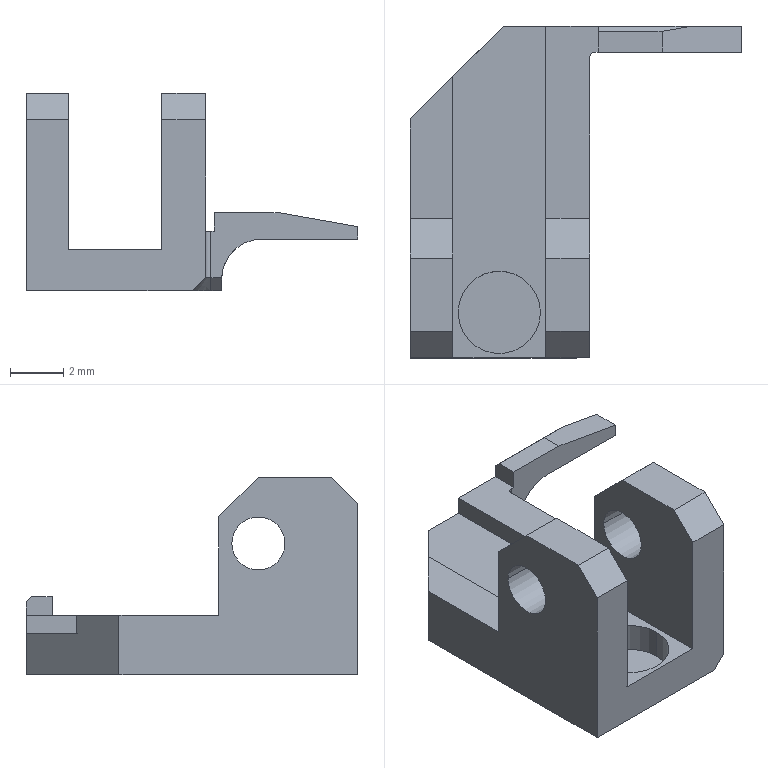Part | NX | 1 solid | 39 faces | box 12.481 x 12.5 x 7.45 mm | volume 216.351 mm3 | plane 30 | cylinder 8 | cone 1 | commonest cylinder face diameters 2 x4 3.1 x2 0.4 x1 3 x1
STEP:
#1=CARTESIAN_POINT('',(-42.479,-42.729,-0.8259));
#2=VERTEX_POINT('',#1);
#3=CARTESIAN_POINT('',(-42.479,-43.716,-0.8259));
#4=VERTEX_POINT('',#3);
#5=CARTESIAN_POINT('',(-42.479,-43.322,-0.8259));
#6=DIRECTION('',(0.,-1.,0.));
#7=VECTOR('',#6,1000.);
#8=LINE('',#5,#7);
#9=EDGE_CURVE('',#2,#4,#8,.T.);
#10=ORIENTED_EDGE('',*,*,#9,.T.);
#11=CARTESIAN_POINT('',(-42.479,-43.716,-1.297));
#12=VERTEX_POINT('',#11);
#13=CARTESIAN_POINT('',(-42.479,-43.716,-2.097));
#14=DIRECTION('',(0.,0.,1.));
#15=VECTOR('',#14,1000.);
#16=LINE('',#13,#15);
#17=EDGE_CURVE('',#12,#4,#16,.T.);
#18=ORIENTED_EDGE('',*,*,#17,.F.);
#19=CARTESIAN_POINT('',(-42.479,-42.729,-1.297));
#20=VERTEX_POINT('',#19);
#21=CARTESIAN_POINT('',(-42.479,-42.161,-1.297));
#22=DIRECTION('',(0.,1.,0.));
#23=VECTOR('',#22,1000.);
#24=LINE('',#21,#23);
#25=EDGE_CURVE('',#12,#20,#24,.T.);
#26=ORIENTED_EDGE('',*,*,#25,.T.);
#27=CARTESIAN_POINT('',(-42.479,-42.729,-2.097));
#28=DIRECTION('',(0.,0.,-1.));
#29=VECTOR('',#28,1000.);
#30=LINE('',#27,#29);
#31=EDGE_CURVE('',#2,#20,#30,.T.);
#32=ORIENTED_EDGE('',*,*,#31,.F.);
#33=EDGE_LOOP('',(#10,#18,#26,#32));
#34=FACE_BOUND('',#33,.T.);
#35=CARTESIAN_POINT('',(-42.479,-43.677,-2.097));
#36=DIRECTION('',(1.,0.,0.));
#37=DIRECTION('',(0.,0.,1.));
#38=AXIS2_PLACEMENT_3D('',#35,#36,#37);
#39=PLANE('',#38);
#40=ADVANCED_FACE('',(#34),#39,.T.);
#41=CARTESIAN_POINT('',(-47.879,-43.716,-0.9969));
#42=VERTEX_POINT('',#41);
#43=CARTESIAN_POINT('',(-47.879,-43.716,-0.2969));
#44=VERTEX_POINT('',#43);
#45=CARTESIAN_POINT('',(-47.879,-43.716,-2.097));
#46=DIRECTION('',(0.,0.,1.));
#47=VECTOR('',#46,1000.);
#48=LINE('',#45,#47);
#49=EDGE_CURVE('',#42,#44,#48,.T.);
#50=ORIENTED_EDGE('',*,*,#49,.T.);
#51=CARTESIAN_POINT('',(-47.879,-42.929,-0.2969));
#52=VERTEX_POINT('',#51);
#53=CARTESIAN_POINT('',(-47.879,-42.161,-0.2969));
#54=DIRECTION('',(0.,-1.,0.));
#55=VECTOR('',#54,1000.);
#56=LINE('',#53,#55);
#57=EDGE_CURVE('',#52,#44,#56,.T.);
#58=ORIENTED_EDGE('',*,*,#57,.F.);
#59=CARTESIAN_POINT('',(-47.879,-42.729,-0.4969));
#60=VERTEX_POINT('',#59);
#61=CARTESIAN_POINT('',(-47.879,-42.161,-1.065));
#62=DIRECTION('',(0.,0.7071,-0.7071));
#63=VECTOR('',#62,1000.);
#64=LINE('',#61,#63);
#65=EDGE_CURVE('',#52,#60,#64,.T.);
#66=ORIENTED_EDGE('',*,*,#65,.T.);
#67=CARTESIAN_POINT('',(-47.879,-42.729,-0.9969));
#68=VERTEX_POINT('',#67);
#69=CARTESIAN_POINT('',(-47.879,-42.729,-2.097));
#70=DIRECTION('',(0.,0.,-1.));
#71=VECTOR('',#70,1000.);
#72=LINE('',#69,#71);
#73=EDGE_CURVE('',#60,#68,#72,.T.);
#74=ORIENTED_EDGE('',*,*,#73,.T.);
#75=CARTESIAN_POINT('',(-47.879,-42.161,-0.9969));
#76=DIRECTION('',(0.,-1.,0.));
#77=VECTOR('',#76,1000.);
#78=LINE('',#75,#77);
#79=EDGE_CURVE('',#68,#42,#78,.T.);
#80=ORIENTED_EDGE('',*,*,#79,.T.);
#81=EDGE_LOOP('',(#50,#58,#66,#74,#80));
#82=FACE_BOUND('',#81,.T.);
#83=CARTESIAN_POINT('',(-47.879,-42.677,-2.097));
#84=DIRECTION('',(-1.,0.,0.));
#85=DIRECTION('',(0.,1.,0.));
#86=AXIS2_PLACEMENT_3D('',#83,#84,#85);
#87=PLANE('',#86);
#88=ADVANCED_FACE('',(#82),#87,.T.);
#89=CARTESIAN_POINT('',(-53.36,-55.229,-1.697));
#90=VERTEX_POINT('',#89);
#91=CARTESIAN_POINT('',(-53.36,-55.229,3.203));
#92=VERTEX_POINT('',#91);
#93=CARTESIAN_POINT('',(-53.36,-55.229,-2.097));
#94=DIRECTION('',(0.,0.,1.));
#95=VECTOR('',#94,1000.);
#96=LINE('',#93,#95);
#97=EDGE_CURVE('',#90,#92,#96,.T.);
#98=ORIENTED_EDGE('',*,*,#97,.F.);
#99=CARTESIAN_POINT('',(-53.36,-44.629,-1.697));
#100=VERTEX_POINT('',#99);
#101=CARTESIAN_POINT('',(-53.36,-42.161,-1.697));
#102=DIRECTION('',(0.,-1.,0.));
#103=VECTOR('',#102,1000.);
#104=LINE('',#101,#103);
#105=EDGE_CURVE('',#100,#90,#104,.T.);
#106=ORIENTED_EDGE('',*,*,#105,.F.);
#107=CARTESIAN_POINT('',(-53.36,-44.629,-0.9969));
#108=VERTEX_POINT('',#107);
#109=CARTESIAN_POINT('',(-53.36,-44.629,-2.097));
#110=DIRECTION('',(0.,0.,-1.));
#111=VECTOR('',#110,1000.);
#112=LINE('',#109,#111);
#113=EDGE_CURVE('',#108,#100,#112,.T.);
#114=ORIENTED_EDGE('',*,*,#113,.F.);
#115=CARTESIAN_POINT('',(-53.36,-49.979,-0.9969));
#116=VERTEX_POINT('',#115);
#117=CARTESIAN_POINT('',(-53.36,-42.161,-0.9969));
#118=DIRECTION('',(0.,-1.,0.));
#119=VECTOR('',#118,1000.);
#120=LINE('',#117,#119);
#121=EDGE_CURVE('',#108,#116,#120,.T.);
#122=ORIENTED_EDGE('',*,*,#121,.T.);
#123=CARTESIAN_POINT('',(-53.36,-49.979,2.703));
#124=VERTEX_POINT('',#123);
#125=CARTESIAN_POINT('',(-53.36,-49.979,-2.097));
#126=DIRECTION('',(0.,0.,-1.));
#127=VECTOR('',#126,1000.);
#128=LINE('',#125,#127);
#129=EDGE_CURVE('',#124,#116,#128,.T.);
#130=ORIENTED_EDGE('',*,*,#129,.F.);
#131=CARTESIAN_POINT('',(-53.36,-51.479,4.203));
#132=VERTEX_POINT('',#131);
#133=CARTESIAN_POINT('',(-53.36,-45.179,-2.097));
#134=DIRECTION('',(0.,-0.7071,0.7071));
#135=VECTOR('',#134,1000.);
#136=LINE('',#133,#135);
#137=EDGE_CURVE('',#124,#132,#136,.T.);
#138=ORIENTED_EDGE('',*,*,#137,.T.);
#139=CARTESIAN_POINT('',(-53.36,-54.229,4.203));
#140=VERTEX_POINT('',#139);
#141=CARTESIAN_POINT('',(-53.36,-42.161,4.203));
#142=DIRECTION('',(0.,1.,0.));
#143=VECTOR('',#142,1000.);
#144=LINE('',#141,#143);
#145=EDGE_CURVE('',#140,#132,#144,.T.);
#146=ORIENTED_EDGE('',*,*,#145,.F.);
#147=CARTESIAN_POINT('',(-53.36,-60.529,-2.097));
#148=DIRECTION('',(0.,-0.7071,-0.7071));
#149=VECTOR('',#148,1000.);
#150=LINE('',#147,#149);
#151=EDGE_CURVE('',#140,#92,#150,.T.);
#152=ORIENTED_EDGE('',*,*,#151,.T.);
#153=EDGE_LOOP('',(#98,#106,#114,#122,#130,#138,#146,#152));
#154=FACE_BOUND('',#153,.T.);
#155=CARTESIAN_POINT('',(-53.36,-50.479,1.703));
#156=VERTEX_POINT('',#155);
#157=CARTESIAN_POINT('',(-53.36,-52.479,1.703));
#158=VERTEX_POINT('',#157);
#159=CARTESIAN_POINT('',(-53.36,-51.479,1.703));
#160=DIRECTION('',(-1.,0.,0.));
#161=DIRECTION('',(0.,-1.,0.));
#162=AXIS2_PLACEMENT_3D('',#159,#160,#161);
#163=CIRCLE('',#162,1.);
#164=EDGE_CURVE('',#156,#158,#163,.T.);
#165=ORIENTED_EDGE('',*,*,#164,.T.);
#166=CARTESIAN_POINT('',(-53.36,-51.479,1.703));
#167=DIRECTION('',(-1.,0.,0.));
#168=DIRECTION('',(0.,-1.,0.));
#169=AXIS2_PLACEMENT_3D('',#166,#167,#168);
#170=CIRCLE('',#169,1.);
#171=EDGE_CURVE('',#158,#156,#170,.T.);
#172=ORIENTED_EDGE('',*,*,#171,.T.);
#173=EDGE_LOOP('',(#165,#172));
#174=FACE_BOUND('',#173,.T.);
#175=CARTESIAN_POINT('',(-53.36,-41.455,-0.9969));
#176=DIRECTION('',(-1.,0.,0.));
#177=DIRECTION('',(0.,0.,1.));
#178=AXIS2_PLACEMENT_3D('',#175,#176,#177);
#179=PLANE('',#178);
#180=ADVANCED_FACE('',(#154,#174),#179,.F.);
#181=ORIENTED_EDGE('',*,*,#31,.T.);
#182=CARTESIAN_POINT('',(-46.102,-42.729,-1.297));
#183=VERTEX_POINT('',#182);
#184=CARTESIAN_POINT('',(-49.458,-42.729,-1.297));
#185=DIRECTION('',(-1.,0.,0.));
#186=VECTOR('',#185,1000.);
#187=LINE('',#184,#186);
#188=EDGE_CURVE('',#20,#183,#187,.T.);
#189=ORIENTED_EDGE('',*,*,#188,.T.);
#190=CARTESIAN_POINT('',(-47.602,-42.729,-2.797));
#191=VERTEX_POINT('',#190);
#192=CARTESIAN_POINT('',(-47.602,-42.729,-2.797));
#193=CARTESIAN_POINT('',(-47.602,-42.729,-2.772));
#194=CARTESIAN_POINT('',(-47.602,-42.729,-2.748));
#195=CARTESIAN_POINT('',(-47.6,-42.729,-2.724));
#196=CARTESIAN_POINT('',(-47.599,-42.729,-2.699));
#197=CARTESIAN_POINT('',(-47.597,-42.729,-2.675));
#198=CARTESIAN_POINT('',(-47.595,-42.729,-2.65));
#199=CARTESIAN_POINT('',(-47.593,-42.729,-2.626));
#200=CARTESIAN_POINT('',(-47.59,-42.729,-2.601));
#201=CARTESIAN_POINT('',(-47.586,-42.729,-2.577));
#202=CARTESIAN_POINT('',(-47.582,-42.729,-2.553));
#203=CARTESIAN_POINT('',(-47.578,-42.729,-2.528));
#204=CARTESIAN_POINT('',(-47.573,-42.729,-2.504));
#205=CARTESIAN_POINT('',(-47.569,-42.729,-2.48));
#206=CARTESIAN_POINT('',(-47.563,-42.729,-2.456));
#207=CARTESIAN_POINT('',(-47.557,-42.729,-2.432));
#208=CARTESIAN_POINT('',(-47.551,-42.729,-2.408));
#209=CARTESIAN_POINT('',(-47.545,-42.729,-2.385));
#210=CARTESIAN_POINT('',(-47.537,-42.729,-2.361));
#211=CARTESIAN_POINT('',(-47.53,-42.729,-2.338));
#212=CARTESIAN_POINT('',(-47.523,-42.729,-2.314));
#213=CARTESIAN_POINT('',(-47.514,-42.729,-2.291));
#214=CARTESIAN_POINT('',(-47.506,-42.729,-2.268));
#215=CARTESIAN_POINT('',(-47.497,-42.729,-2.245));
#216=CARTESIAN_POINT('',(-47.488,-42.729,-2.223));
#217=CARTESIAN_POINT('',(-47.479,-42.729,-2.2));
#218=CARTESIAN_POINT('',(-47.469,-42.729,-2.178));
#219=CARTESIAN_POINT('',(-47.458,-42.729,-2.156));
#220=CARTESIAN_POINT('',(-47.448,-42.729,-2.134));
#221=CARTESIAN_POINT('',(-47.437,-42.729,-2.112));
#222=CARTESIAN_POINT('',(-47.425,-42.729,-2.09));
#223=CARTESIAN_POINT('',(-47.414,-42.729,-2.068));
#224=CARTESIAN_POINT('',(-47.401,-42.729,-2.047));
#225=CARTESIAN_POINT('',(-47.389,-42.729,-2.026));
#226=CARTESIAN_POINT('',(-47.376,-42.729,-2.005));
#227=CARTESIAN_POINT('',(-47.363,-42.729,-1.984));
#228=CARTESIAN_POINT('',(-47.349,-42.729,-1.963));
#229=CARTESIAN_POINT('',(-47.336,-42.729,-1.943));
#230=CARTESIAN_POINT('',(-47.321,-42.729,-1.923));
#231=CARTESIAN_POINT('',(-47.307,-42.729,-1.903));
#232=CARTESIAN_POINT('',(-47.292,-42.729,-1.883));
#233=CARTESIAN_POINT('',(-47.277,-42.729,-1.864));
#234=CARTESIAN_POINT('',(-47.261,-42.729,-1.845));
#235=CARTESIAN_POINT('',(-47.246,-42.729,-1.826));
#236=CARTESIAN_POINT('',(-47.23,-42.729,-1.807));
#237=CARTESIAN_POINT('',(-47.213,-42.729,-1.789));
#238=CARTESIAN_POINT('',(-47.197,-42.729,-1.771));
#239=CARTESIAN_POINT('',(-47.18,-42.729,-1.753));
#240=CARTESIAN_POINT('',(-47.163,-42.729,-1.736));
#241=CARTESIAN_POINT('',(-47.145,-42.729,-1.719));
#242=CARTESIAN_POINT('',(-47.128,-42.729,-1.702));
#243=CARTESIAN_POINT('',(-47.11,-42.729,-1.686));
#244=CARTESIAN_POINT('',(-47.091,-42.729,-1.669));
#245=CARTESIAN_POINT('',(-47.073,-42.729,-1.653));
#246=CARTESIAN_POINT('',(-47.054,-42.729,-1.638));
#247=CARTESIAN_POINT('',(-47.035,-42.729,-1.622));
#248=CARTESIAN_POINT('',(-47.016,-42.729,-1.607));
#249=CARTESIAN_POINT('',(-46.996,-42.729,-1.592));
#250=CARTESIAN_POINT('',(-46.976,-42.729,-1.577));
#251=CARTESIAN_POINT('',(-46.956,-42.729,-1.563));
#252=CARTESIAN_POINT('',(-46.935,-42.729,-1.55));
#253=CARTESIAN_POINT('',(-46.915,-42.729,-1.536));
#254=CARTESIAN_POINT('',(-46.894,-42.729,-1.523));
#255=CARTESIAN_POINT('',(-46.873,-42.729,-1.51));
#256=CARTESIAN_POINT('',(-46.852,-42.729,-1.497));
#257=CARTESIAN_POINT('',(-46.83,-42.729,-1.485));
#258=CARTESIAN_POINT('',(-46.809,-42.729,-1.474));
#259=CARTESIAN_POINT('',(-46.787,-42.729,-1.462));
#260=CARTESIAN_POINT('',(-46.765,-42.729,-1.451));
#261=CARTESIAN_POINT('',(-46.743,-42.729,-1.441));
#262=CARTESIAN_POINT('',(-46.721,-42.729,-1.43));
#263=CARTESIAN_POINT('',(-46.698,-42.729,-1.42));
#264=CARTESIAN_POINT('',(-46.676,-42.729,-1.411));
#265=CARTESIAN_POINT('',(-46.631,-42.729,-1.392));
#266=CARTESIAN_POINT('',(-46.585,-42.729,-1.376));
#267=CARTESIAN_POINT('',(-46.538,-42.729,-1.362));
#268=CARTESIAN_POINT('',(-46.514,-42.729,-1.354));
#269=CARTESIAN_POINT('',(-46.491,-42.729,-1.348));
#270=CARTESIAN_POINT('',(-46.467,-42.729,-1.342));
#271=CARTESIAN_POINT('',(-46.443,-42.729,-1.336));
#272=CARTESIAN_POINT('',(-46.419,-42.729,-1.33));
#273=CARTESIAN_POINT('',(-46.395,-42.729,-1.326));
#274=CARTESIAN_POINT('',(-46.371,-42.729,-1.321));
#275=CARTESIAN_POINT('',(-46.346,-42.729,-1.317));
#276=CARTESIAN_POINT('',(-46.322,-42.729,-1.313));
#277=CARTESIAN_POINT('',(-46.298,-42.729,-1.309));
#278=CARTESIAN_POINT('',(-46.273,-42.729,-1.306));
#279=CARTESIAN_POINT('',(-46.249,-42.729,-1.304));
#280=CARTESIAN_POINT('',(-46.224,-42.729,-1.302));
#281=CARTESIAN_POINT('',(-46.2,-42.729,-1.3));
#282=CARTESIAN_POINT('',(-46.175,-42.729,-1.299));
#283=CARTESIAN_POINT('',(-46.151,-42.729,-1.297));
#284=CARTESIAN_POINT('',(-46.127,-42.729,-1.297));
#285=CARTESIAN_POINT('',(-46.102,-42.729,-1.297));
#286=B_SPLINE_CURVE_WITH_KNOTS('',3,(#192,#193,#194,#195,#196,#197,#198,#199,#200,#201,#202,#203,#204,#205,#206,#207,#208,#209,#210,#211,#212,#213,#214,#215,#216,#217,#218,#219,#220,#221,#222,#223,#224,#225,#226,#227,#228,#229,#230,#231,#232,#233,#234,#235,#236,#237,#238,#239,#240,#241,#242,#243,#244,#245,#246,#247,#248,#249,#250,#251,#252,#253,#254,#255,#256,#257,#258,#259,#260,#261,#262,#263,#264,#265,#266,#267,#268,#269,#270,#271,#272,#273,#274,#275,#276,#277,#278,#279,#280,#281,#282,#283,#284,#285),.UNSPECIFIED.,.F.,.F.,(4,3,3,3,3,3,3,3,3,3,3,3,3,3,3,3,3,3,3,3,3,3,3,3,3,3,3,3,3,3,3,4),(0.,0.07332,0.1469,0.2207,0.2945,0.3684,0.4422,0.5158,0.5891,0.6624,0.736,0.8098,0.8836,0.9575,1.031,1.105,1.178,1.252,1.325,1.399,1.473,1.547,1.62,1.694,1.767,1.914,1.988,2.062,2.136,2.209,2.283,2.356),.UNSPECIFIED.);
#287=EDGE_CURVE('',#191,#183,#286,.T.);
#288=ORIENTED_EDGE('',*,*,#287,.F.);
#289=CARTESIAN_POINT('',(-47.602,-42.729,-3.247));
#290=VERTEX_POINT('',#289);
#291=CARTESIAN_POINT('',(-47.602,-42.729,-2.097));
#292=DIRECTION('',(0.,0.,1.));
#293=VECTOR('',#292,1000.);
#294=LINE('',#291,#293);
#295=EDGE_CURVE('',#290,#191,#294,.T.);
#296=ORIENTED_EDGE('',*,*,#295,.F.);
#297=CARTESIAN_POINT('',(-51.46,-42.729,-3.247));
#298=VERTEX_POINT('',#297);
#299=CARTESIAN_POINT('',(-49.458,-42.729,-3.247));
#300=DIRECTION('',(-1.,0.,0.));
#301=VECTOR('',#300,1000.);
#302=LINE('',#299,#301);
#303=EDGE_CURVE('',#290,#298,#302,.T.);
#304=ORIENTED_EDGE('',*,*,#303,.T.);
#305=CARTESIAN_POINT('',(-51.46,-42.729,-1.697));
#306=VERTEX_POINT('',#305);
#307=CARTESIAN_POINT('',(-51.46,-42.729,-2.097));
#308=DIRECTION('',(0.,0.,1.));
#309=VECTOR('',#308,1000.);
#310=LINE('',#307,#309);
#311=EDGE_CURVE('',#298,#306,#310,.T.);
#312=ORIENTED_EDGE('',*,*,#311,.T.);
#313=CARTESIAN_POINT('',(-49.86,-42.729,-1.697));
#314=VERTEX_POINT('',#313);
#315=CARTESIAN_POINT('',(-49.458,-42.729,-1.697));
#316=DIRECTION('',(-1.,0.,0.));
#317=VECTOR('',#316,1000.);
#318=LINE('',#315,#317);
#319=EDGE_CURVE('',#314,#306,#318,.T.);
#320=ORIENTED_EDGE('',*,*,#319,.F.);
#321=CARTESIAN_POINT('',(-49.86,-42.729,-0.9969));
#322=VERTEX_POINT('',#321);
#323=CARTESIAN_POINT('',(-49.86,-42.729,-2.097));
#324=DIRECTION('',(0.,0.,-1.));
#325=VECTOR('',#324,1000.);
#326=LINE('',#323,#325);
#327=EDGE_CURVE('',#322,#314,#326,.T.);
#328=ORIENTED_EDGE('',*,*,#327,.F.);
#329=CARTESIAN_POINT('',(-49.458,-42.729,-0.9969));
#330=DIRECTION('',(-1.,0.,0.));
#331=VECTOR('',#330,1000.);
#332=LINE('',#329,#331);
#333=EDGE_CURVE('',#68,#322,#332,.T.);
#334=ORIENTED_EDGE('',*,*,#333,.F.);
#335=ORIENTED_EDGE('',*,*,#73,.F.);
#336=CARTESIAN_POINT('',(-44.345,-42.729,-0.4969));
#337=VERTEX_POINT('',#336);
#338=CARTESIAN_POINT('',(-49.458,-42.729,-0.4969));
#339=DIRECTION('',(1.,0.,0.));
#340=VECTOR('',#339,1000.);
#341=LINE('',#338,#340);
#342=EDGE_CURVE('',#60,#337,#341,.T.);
#343=ORIENTED_EDGE('',*,*,#342,.T.);
#344=CARTESIAN_POINT('',(-49.458,-42.729,0.4047));
#345=DIRECTION('',(0.9848,0.,-0.1736));
#346=VECTOR('',#345,1000.);
#347=LINE('',#344,#346);
#348=EDGE_CURVE('',#337,#2,#347,.T.);
#349=ORIENTED_EDGE('',*,*,#348,.T.);
#350=EDGE_LOOP('',(#181,#189,#288,#296,#304,#312,#320,#328,#334,#335,#343,#349));
#351=FACE_BOUND('',#350,.T.);
#352=CARTESIAN_POINT('',(-40.479,-42.729,-2.097));
#353=DIRECTION('',(0.,1.,0.));
#354=DIRECTION('',(0.,0.,-1.));
#355=AXIS2_PLACEMENT_3D('',#352,#353,#354);
#356=PLANE('',#355);
#357=ADVANCED_FACE('',(#351),#356,.T.);
#358=CARTESIAN_POINT('',(-48.01,-43.716,-2.747));
#359=VERTEX_POINT('',#358);
#360=CARTESIAN_POINT('',(-47.601,-43.716,-2.747));
#361=VERTEX_POINT('',#360);
#362=CARTESIAN_POINT('',(-47.806,-43.716,-2.747));
#363=DIRECTION('',(1.,0.,0.));
#364=VECTOR('',#363,1000.);
#365=LINE('',#362,#364);
#366=EDGE_CURVE('',#359,#361,#365,.T.);
#367=ORIENTED_EDGE('',*,*,#366,.T.);
#368=CARTESIAN_POINT('',(-46.102,-43.716,-1.297));
#369=VERTEX_POINT('',#368);
#370=CARTESIAN_POINT('',(-46.102,-43.716,-1.297));
#371=CARTESIAN_POINT('',(-46.126,-43.716,-1.297));
#372=CARTESIAN_POINT('',(-46.15,-43.716,-1.297));
#373=CARTESIAN_POINT('',(-46.174,-43.716,-1.299));
#374=CARTESIAN_POINT('',(-46.198,-43.716,-1.3));
#375=CARTESIAN_POINT('',(-46.222,-43.716,-1.301));
#376=CARTESIAN_POINT('',(-46.246,-43.716,-1.304));
#377=CARTESIAN_POINT('',(-46.27,-43.716,-1.306));
#378=CARTESIAN_POINT('',(-46.294,-43.716,-1.309));
#379=CARTESIAN_POINT('',(-46.317,-43.716,-1.312));
#380=CARTESIAN_POINT('',(-46.341,-43.716,-1.316));
#381=CARTESIAN_POINT('',(-46.365,-43.716,-1.32));
#382=CARTESIAN_POINT('',(-46.389,-43.716,-1.324));
#383=CARTESIAN_POINT('',(-46.412,-43.716,-1.329));
#384=CARTESIAN_POINT('',(-46.436,-43.716,-1.334));
#385=CARTESIAN_POINT('',(-46.459,-43.716,-1.34));
#386=CARTESIAN_POINT('',(-46.483,-43.716,-1.346));
#387=CARTESIAN_POINT('',(-46.506,-43.716,-1.352));
#388=CARTESIAN_POINT('',(-46.529,-43.716,-1.359));
#389=CARTESIAN_POINT('',(-46.552,-43.716,-1.366));
#390=CARTESIAN_POINT('',(-46.575,-43.716,-1.373));
#391=CARTESIAN_POINT('',(-46.597,-43.716,-1.381));
#392=CARTESIAN_POINT('',(-46.62,-43.716,-1.389));
#393=CARTESIAN_POINT('',(-46.643,-43.716,-1.397));
#394=CARTESIAN_POINT('',(-46.665,-43.716,-1.406));
#395=CARTESIAN_POINT('',(-46.709,-43.716,-1.424));
#396=CARTESIAN_POINT('',(-46.752,-43.716,-1.444));
#397=CARTESIAN_POINT('',(-46.795,-43.716,-1.467));
#398=CARTESIAN_POINT('',(-46.816,-43.716,-1.478));
#399=CARTESIAN_POINT('',(-46.837,-43.716,-1.489));
#400=CARTESIAN_POINT('',(-46.858,-43.716,-1.501));
#401=CARTESIAN_POINT('',(-46.879,-43.716,-1.514));
#402=CARTESIAN_POINT('',(-46.9,-43.716,-1.526));
#403=CARTESIAN_POINT('',(-46.92,-43.716,-1.539));
#404=CARTESIAN_POINT('',(-46.94,-43.716,-1.552));
#405=CARTESIAN_POINT('',(-46.96,-43.716,-1.566));
#406=CARTESIAN_POINT('',(-46.979,-43.716,-1.58));
#407=CARTESIAN_POINT('',(-46.999,-43.716,-1.594));
#408=CARTESIAN_POINT('',(-47.018,-43.716,-1.609));
#409=CARTESIAN_POINT('',(-47.037,-43.716,-1.624));
#410=CARTESIAN_POINT('',(-47.056,-43.716,-1.639));
#411=CARTESIAN_POINT('',(-47.074,-43.716,-1.654));
#412=CARTESIAN_POINT('',(-47.092,-43.716,-1.67));
#413=CARTESIAN_POINT('',(-47.11,-43.716,-1.686));
#414=CARTESIAN_POINT('',(-47.128,-43.716,-1.702));
#415=CARTESIAN_POINT('',(-47.145,-43.716,-1.719));
#416=CARTESIAN_POINT('',(-47.162,-43.716,-1.735));
#417=CARTESIAN_POINT('',(-47.179,-43.716,-1.752));
#418=CARTESIAN_POINT('',(-47.195,-43.716,-1.77));
#419=CARTESIAN_POINT('',(-47.212,-43.716,-1.787));
#420=CARTESIAN_POINT('',(-47.228,-43.716,-1.805));
#421=CARTESIAN_POINT('',(-47.243,-43.716,-1.823));
#422=CARTESIAN_POINT('',(-47.259,-43.716,-1.842));
#423=CARTESIAN_POINT('',(-47.274,-43.716,-1.86));
#424=CARTESIAN_POINT('',(-47.289,-43.716,-1.879));
#425=CARTESIAN_POINT('',(-47.304,-43.716,-1.898));
#426=CARTESIAN_POINT('',(-47.318,-43.716,-1.918));
#427=CARTESIAN_POINT('',(-47.332,-43.716,-1.938));
#428=CARTESIAN_POINT('',(-47.345,-43.716,-1.957));
#429=CARTESIAN_POINT('',(-47.359,-43.716,-1.977));
#430=CARTESIAN_POINT('',(-47.372,-43.716,-1.998));
#431=CARTESIAN_POINT('',(-47.384,-43.716,-2.018));
#432=CARTESIAN_POINT('',(-47.397,-43.716,-2.039));
#433=CARTESIAN_POINT('',(-47.409,-43.716,-2.06));
#434=CARTESIAN_POINT('',(-47.42,-43.716,-2.081));
#435=CARTESIAN_POINT('',(-47.432,-43.716,-2.102));
#436=CARTESIAN_POINT('',(-47.443,-43.716,-2.124));
#437=CARTESIAN_POINT('',(-47.453,-43.716,-2.145));
#438=CARTESIAN_POINT('',(-47.464,-43.716,-2.167));
#439=CARTESIAN_POINT('',(-47.473,-43.716,-2.189));
#440=CARTESIAN_POINT('',(-47.483,-43.716,-2.21));
#441=CARTESIAN_POINT('',(-47.492,-43.716,-2.233));
#442=CARTESIAN_POINT('',(-47.501,-43.716,-2.255));
#443=CARTESIAN_POINT('',(-47.509,-43.716,-2.277));
#444=CARTESIAN_POINT('',(-47.518,-43.716,-2.3));
#445=CARTESIAN_POINT('',(-47.525,-43.716,-2.322));
#446=CARTESIAN_POINT('',(-47.533,-43.716,-2.345));
#447=CARTESIAN_POINT('',(-47.54,-43.716,-2.368));
#448=CARTESIAN_POINT('',(-47.546,-43.716,-2.391));
#449=CARTESIAN_POINT('',(-47.553,-43.716,-2.414));
#450=CARTESIAN_POINT('',(-47.559,-43.716,-2.438));
#451=CARTESIAN_POINT('',(-47.564,-43.716,-2.461));
#452=CARTESIAN_POINT('',(-47.569,-43.716,-2.485));
#453=CARTESIAN_POINT('',(-47.574,-43.716,-2.508));
#454=CARTESIAN_POINT('',(-47.579,-43.716,-2.532));
#455=CARTESIAN_POINT('',(-47.583,-43.716,-2.556));
#456=CARTESIAN_POINT('',(-47.587,-43.716,-2.579));
#457=CARTESIAN_POINT('',(-47.59,-43.716,-2.603));
#458=CARTESIAN_POINT('',(-47.593,-43.716,-2.627));
#459=CARTESIAN_POINT('',(-47.595,-43.716,-2.651));
#460=CARTESIAN_POINT('',(-47.597,-43.716,-2.675));
#461=CARTESIAN_POINT('',(-47.599,-43.716,-2.699));
#462=CARTESIAN_POINT('',(-47.601,-43.716,-2.723));
#463=CARTESIAN_POINT('',(-47.601,-43.716,-2.747));
#464=B_SPLINE_CURVE_WITH_KNOTS('',3,(#370,#371,#372,#373,#374,#375,#376,#377,#378,#379,#380,#381,#382,#383,#384,#385,#386,#387,#388,#389,#390,#391,#392,#393,#394,#395,#396,#397,#398,#399,#400,#401,#402,#403,#404,#405,#406,#407,#408,#409,#410,#411,#412,#413,#414,#415,#416,#417,#418,#419,#420,#421,#422,#423,#424,#425,#426,#427,#428,#429,#430,#431,#432,#433,#434,#435,#436,#437,#438,#439,#440,#441,#442,#443,#444,#445,#446,#447,#448,#449,#450,#451,#452,#453,#454,#455,#456,#457,#458,#459,#460,#461,#462,#463),.UNSPECIFIED.,.F.,.F.,(4,3,3,3,3,3,3,3,3,3,3,3,3,3,3,3,3,3,3,3,3,3,3,3,3,3,3,3,3,3,3,4),(0.,0.07175,0.1438,0.216,0.2882,0.3605,0.4328,0.5048,0.5766,0.7203,0.7924,0.8647,0.937,1.009,1.081,1.153,1.225,1.297,1.369,1.441,1.514,1.586,1.658,1.73,1.802,1.873,1.945,2.018,2.09,2.162,2.234,2.306),.UNSPECIFIED.);
#465=EDGE_CURVE('',#369,#361,#464,.T.);
#466=ORIENTED_EDGE('',*,*,#465,.F.);
#467=CARTESIAN_POINT('',(-49.458,-43.716,-1.297));
#468=DIRECTION('',(1.,0.,0.));
#469=VECTOR('',#468,1000.);
#470=LINE('',#467,#469);
#471=EDGE_CURVE('',#369,#12,#470,.T.);
#472=ORIENTED_EDGE('',*,*,#471,.T.);
#473=ORIENTED_EDGE('',*,*,#17,.T.);
#474=CARTESIAN_POINT('',(-45.479,-43.716,-0.2969));
#475=VERTEX_POINT('',#474);
#476=CARTESIAN_POINT('',(-49.458,-43.716,0.4047));
#477=DIRECTION('',(-0.9848,0.,0.1736));
#478=VECTOR('',#477,1000.);
#479=LINE('',#476,#478);
#480=EDGE_CURVE('',#4,#475,#479,.T.);
#481=ORIENTED_EDGE('',*,*,#480,.T.);
#482=CARTESIAN_POINT('',(-49.458,-43.716,-0.2969));
#483=DIRECTION('',(-1.,0.,0.));
#484=VECTOR('',#483,1000.);
#485=LINE('',#482,#484);
#486=EDGE_CURVE('',#475,#44,#485,.T.);
#487=ORIENTED_EDGE('',*,*,#486,.T.);
#488=ORIENTED_EDGE('',*,*,#49,.F.);
#489=CARTESIAN_POINT('',(-48.01,-43.716,-0.9969));
#490=VERTEX_POINT('',#489);
#491=CARTESIAN_POINT('',(-49.458,-43.716,-0.9969));
#492=DIRECTION('',(1.,0.,0.));
#493=VECTOR('',#492,1000.);
#494=LINE('',#491,#493);
#495=EDGE_CURVE('',#490,#42,#494,.T.);
#496=ORIENTED_EDGE('',*,*,#495,.F.);
#497=CARTESIAN_POINT('',(-48.01,-43.716,-2.097));
#498=DIRECTION('',(0.,0.,-1.));
#499=VECTOR('',#498,1000.);
#500=LINE('',#497,#499);
#501=EDGE_CURVE('',#490,#359,#500,.T.);
#502=ORIENTED_EDGE('',*,*,#501,.T.);
#503=EDGE_LOOP('',(#367,#466,#472,#473,#481,#487,#488,#496,#502));
#504=FACE_BOUND('',#503,.T.);
#505=CARTESIAN_POINT('',(-49.857,-43.716,-2.975));
#506=DIRECTION('',(0.,-1.,0.));
#507=DIRECTION('',(-1.,0.,0.));
#508=AXIS2_PLACEMENT_3D('',#505,#506,#507);
#509=PLANE('',#508);
#510=ADVANCED_FACE('',(#504),#509,.T.);
#511=CARTESIAN_POINT('',(-48.21,-55.229,-2.747));
#512=VERTEX_POINT('',#511);
#513=CARTESIAN_POINT('',(-48.21,-55.229,3.203));
#514=VERTEX_POINT('',#513);
#515=CARTESIAN_POINT('',(-48.21,-55.229,-2.097));
#516=DIRECTION('',(0.,0.,1.));
#517=VECTOR('',#516,1000.);
#518=LINE('',#515,#517);
#519=EDGE_CURVE('',#512,#514,#518,.T.);
#520=ORIENTED_EDGE('',*,*,#519,.T.);
#521=CARTESIAN_POINT('',(-49.86,-55.229,3.203));
#522=VERTEX_POINT('',#521);
#523=CARTESIAN_POINT('',(-49.035,-55.229,3.203));
#524=DIRECTION('',(1.,0.,0.));
#525=VECTOR('',#524,1000.);
#526=LINE('',#523,#525);
#527=EDGE_CURVE('',#522,#514,#526,.T.);
#528=ORIENTED_EDGE('',*,*,#527,.F.);
#529=CARTESIAN_POINT('',(-49.86,-55.229,-1.697));
#530=VERTEX_POINT('',#529);
#531=CARTESIAN_POINT('',(-49.86,-55.229,-2.097));
#532=DIRECTION('',(0.,0.,-1.));
#533=VECTOR('',#532,1000.);
#534=LINE('',#531,#533);
#535=EDGE_CURVE('',#522,#530,#534,.T.);
#536=ORIENTED_EDGE('',*,*,#535,.T.);
#537=CARTESIAN_POINT('',(-49.458,-55.229,-1.697));
#538=DIRECTION('',(-1.,0.,0.));
#539=VECTOR('',#538,1000.);
#540=LINE('',#537,#539);
#541=EDGE_CURVE('',#530,#90,#540,.T.);
#542=ORIENTED_EDGE('',*,*,#541,.T.);
#543=ORIENTED_EDGE('',*,*,#97,.T.);
#544=CARTESIAN_POINT('',(-54.96,-55.229,3.203));
#545=VERTEX_POINT('',#544);
#546=CARTESIAN_POINT('',(-54.16,-55.229,3.203));
#547=DIRECTION('',(1.,0.,0.));
#548=VECTOR('',#547,1000.);
#549=LINE('',#546,#548);
#550=EDGE_CURVE('',#545,#92,#549,.T.);
#551=ORIENTED_EDGE('',*,*,#550,.F.);
#552=CARTESIAN_POINT('',(-54.96,-55.229,-3.247));
#553=VERTEX_POINT('',#552);
#554=CARTESIAN_POINT('',(-54.96,-55.229,-2.097));
#555=DIRECTION('',(0.,0.,1.));
#556=VECTOR('',#555,1000.);
#557=LINE('',#554,#556);
#558=EDGE_CURVE('',#553,#545,#557,.T.);
#559=ORIENTED_EDGE('',*,*,#558,.F.);
#560=CARTESIAN_POINT('',(-48.71,-55.229,-3.247));
#561=VERTEX_POINT('',#560);
#562=CARTESIAN_POINT('',(-49.458,-55.229,-3.247));
#563=DIRECTION('',(-1.,0.,0.));
#564=VECTOR('',#563,1000.);
#565=LINE('',#562,#564);
#566=EDGE_CURVE('',#561,#553,#565,.T.);
#567=ORIENTED_EDGE('',*,*,#566,.F.);
#568=CARTESIAN_POINT('',(-49.458,-55.229,-3.995));
#569=DIRECTION('',(-0.7071,0.,-0.7071));
#570=VECTOR('',#569,1000.);
#571=LINE('',#568,#570);
#572=EDGE_CURVE('',#512,#561,#571,.T.);
#573=ORIENTED_EDGE('',*,*,#572,.F.);
#574=EDGE_LOOP('',(#520,#528,#536,#542,#543,#551,#559,#567,#573));
#575=FACE_BOUND('',#574,.T.);
#576=CARTESIAN_POINT('',(-46.479,-55.229,-2.097));
#577=DIRECTION('',(0.,-1.,0.));
#578=DIRECTION('',(-1.,0.,0.));
#579=AXIS2_PLACEMENT_3D('',#576,#577,#578);
#580=PLANE('',#579);
#581=ADVANCED_FACE('',(#575),#580,.T.);
#582=CARTESIAN_POINT('',(-47.602,-43.666,-2.797));
#583=VERTEX_POINT('',#582);
#584=CARTESIAN_POINT('',(-47.602,-43.666,-2.797));
#585=CARTESIAN_POINT('',(-47.602,-43.518,-2.797));
#586=CARTESIAN_POINT('',(-47.602,-43.37,-2.797));
#587=CARTESIAN_POINT('',(-47.602,-43.058,-2.797));
#588=CARTESIAN_POINT('',(-47.602,-42.893,-2.797));
#589=CARTESIAN_POINT('',(-47.602,-42.729,-2.797));
#590=B_SPLINE_CURVE_WITH_KNOTS('',3,(#584,#585,#586,#587,#588,#589),.UNSPECIFIED.,.F.,.F.,(4,2,4),(17.155,17.598,18.092),.UNSPECIFIED.);
#591=EDGE_CURVE('',#583,#191,#590,.T.);
#592=ORIENTED_EDGE('',*,*,#591,.F.);
#593=CARTESIAN_POINT('',(-47.602,-43.216,-3.247));
#594=VERTEX_POINT('',#593);
#595=CARTESIAN_POINT('',(-47.602,-44.366,-2.097));
#596=DIRECTION('',(0.,0.7071,-0.7071));
#597=VECTOR('',#596,1000.);
#598=LINE('',#595,#597);
#599=EDGE_CURVE('',#583,#594,#598,.T.);
#600=ORIENTED_EDGE('',*,*,#599,.T.);
#601=CARTESIAN_POINT('',(-47.602,-42.161,-3.247));
#602=DIRECTION('',(0.,-1.,0.));
#603=VECTOR('',#602,1000.);
#604=LINE('',#601,#603);
#605=EDGE_CURVE('',#290,#594,#604,.T.);
#606=ORIENTED_EDGE('',*,*,#605,.F.);
#607=ORIENTED_EDGE('',*,*,#295,.T.);
#608=EDGE_LOOP('',(#592,#600,#606,#607));
#609=FACE_BOUND('',#608,.T.);
#610=CARTESIAN_POINT('',(-47.602,-42.161,-2.747));
#611=DIRECTION('',(-1.,0.,0.));
#612=DIRECTION('',(0.,0.,1.));
#613=AXIS2_PLACEMENT_3D('',#610,#611,#612);
#614=PLANE('',#613);
#615=ADVANCED_FACE('',(#609),#614,.F.);
#616=ORIENTED_EDGE('',*,*,#591,.T.);
#617=ORIENTED_EDGE('',*,*,#287,.T.);
#618=CARTESIAN_POINT('',(-46.102,-43.716,-1.297));
#619=CARTESIAN_POINT('',(-46.102,-43.551,-1.297));
#620=CARTESIAN_POINT('',(-46.102,-43.387,-1.297));
#621=CARTESIAN_POINT('',(-46.102,-43.058,-1.297));
#622=CARTESIAN_POINT('',(-46.102,-42.893,-1.297));
#623=CARTESIAN_POINT('',(-46.102,-42.729,-1.297));
#624=B_SPLINE_CURVE_WITH_KNOTS('',3,(#618,#619,#620,#621,#622,#623),.UNSPECIFIED.,.F.,.F.,(4,2,4),(17.105,17.598,18.092),.UNSPECIFIED.);
#625=EDGE_CURVE('',#369,#183,#624,.T.);
#626=ORIENTED_EDGE('',*,*,#625,.F.);
#627=ORIENTED_EDGE('',*,*,#465,.T.);
#628=CARTESIAN_POINT('',(-47.602,-43.666,-2.797));
#629=CARTESIAN_POINT('',(-47.602,-43.67,-2.793));
#630=CARTESIAN_POINT('',(-47.602,-43.674,-2.789));
#631=CARTESIAN_POINT('',(-47.602,-43.678,-2.784));
#632=CARTESIAN_POINT('',(-47.602,-43.683,-2.78));
#633=CARTESIAN_POINT('',(-47.602,-43.687,-2.776));
#634=CARTESIAN_POINT('',(-47.602,-43.691,-2.772));
#635=CARTESIAN_POINT('',(-47.602,-43.695,-2.768));
#636=CARTESIAN_POINT('',(-47.602,-43.699,-2.764));
#637=CARTESIAN_POINT('',(-47.602,-43.703,-2.759));
#638=CARTESIAN_POINT('',(-47.602,-43.708,-2.755));
#639=CARTESIAN_POINT('',(-47.601,-43.712,-2.751));
#640=CARTESIAN_POINT('',(-47.601,-43.716,-2.747));
#641=B_SPLINE_CURVE_WITH_KNOTS('',3,(#628,#629,#630,#631,#632,#633,#634,#635,#636,#637,#638,#639,#640),.UNSPECIFIED.,.F.,.F.,(4,3,3,3,4),(0.,0.01766,0.03534,0.05302,0.07072),.UNSPECIFIED.);
#642=EDGE_CURVE('',#583,#361,#641,.T.);
#643=ORIENTED_EDGE('',*,*,#642,.F.);
#644=EDGE_LOOP('',(#616,#617,#626,#627,#643));
#645=FACE_BOUND('',#644,.T.);
#646=CARTESIAN_POINT('',(-46.102,-43.222,-2.797));
#647=DIRECTION('',(0.,1.,0.));
#648=DIRECTION('',(-1.,0.,0.));
#649=AXIS2_PLACEMENT_3D('',#646,#647,#648);
#650=CYLINDRICAL_SURFACE('',#649,1.5);
#651=ADVANCED_FACE('',(#645),#650,.F.);
#652=CARTESIAN_POINT('',(-48.21,-43.916,-2.747));
#653=VERTEX_POINT('',#652);
#654=CARTESIAN_POINT('',(-48.01,-43.916,-2.747));
#655=DIRECTION('',(0.,0.,-1.));
#656=DIRECTION('',(-1.,0.,0.));
#657=AXIS2_PLACEMENT_3D('',#654,#655,#656);
#658=CIRCLE('',#657,0.2);
#659=EDGE_CURVE('',#653,#359,#658,.T.);
#660=ORIENTED_EDGE('',*,*,#659,.T.);
#661=ORIENTED_EDGE('',*,*,#501,.F.);
#662=CARTESIAN_POINT('',(-48.21,-43.916,-0.9969));
#663=VERTEX_POINT('',#662);
#664=CARTESIAN_POINT('',(-48.01,-43.916,-0.9969));
#665=DIRECTION('',(0.,0.,-1.));
#666=DIRECTION('',(-1.,0.,0.));
#667=AXIS2_PLACEMENT_3D('',#664,#665,#666);
#668=CIRCLE('',#667,0.2);
#669=EDGE_CURVE('',#663,#490,#668,.T.);
#670=ORIENTED_EDGE('',*,*,#669,.F.);
#671=CARTESIAN_POINT('',(-48.21,-43.916,-2.097));
#672=DIRECTION('',(0.,0.,-1.));
#673=VECTOR('',#672,1000.);
#674=LINE('',#671,#673);
#675=EDGE_CURVE('',#663,#653,#674,.T.);
#676=ORIENTED_EDGE('',*,*,#675,.T.);
#677=EDGE_LOOP('',(#660,#661,#670,#676));
#678=FACE_BOUND('',#677,.T.);
#679=CARTESIAN_POINT('',(-48.01,-43.916,-2.097));
#680=DIRECTION('',(0.,0.,-1.));
#681=DIRECTION('',(-1.,0.,0.));
#682=AXIS2_PLACEMENT_3D('',#679,#680,#681);
#683=CYLINDRICAL_SURFACE('',#682,0.2);
#684=ADVANCED_FACE('',(#678),#683,.F.);
#685=ORIENTED_EDGE('',*,*,#164,.F.);
#686=CARTESIAN_POINT('',(-54.96,-50.479,1.703));
#687=VERTEX_POINT('',#686);
#688=CARTESIAN_POINT('',(-40.131,-50.479,1.703));
#689=DIRECTION('',(-1.,0.,0.));
#690=VECTOR('',#689,1000.);
#691=LINE('',#688,#690);
#692=EDGE_CURVE('',#687,#156,#691,.F.);
#693=ORIENTED_EDGE('',*,*,#692,.F.);
#694=CARTESIAN_POINT('',(-54.96,-52.479,1.703));
#695=VERTEX_POINT('',#694);
#696=CARTESIAN_POINT('',(-54.96,-51.479,1.703));
#697=DIRECTION('',(-1.,0.,0.));
#698=DIRECTION('',(0.,-1.,0.));
#699=AXIS2_PLACEMENT_3D('',#696,#697,#698);
#700=CIRCLE('',#699,1.);
#701=EDGE_CURVE('',#687,#695,#700,.T.);
#702=ORIENTED_EDGE('',*,*,#701,.T.);
#703=CARTESIAN_POINT('',(-40.131,-52.479,1.703));
#704=DIRECTION('',(-1.,0.,0.));
#705=VECTOR('',#704,1000.);
#706=LINE('',#703,#705);
#707=EDGE_CURVE('',#695,#158,#706,.F.);
#708=ORIENTED_EDGE('',*,*,#707,.T.);
#709=EDGE_LOOP('',(#685,#693,#702,#708));
#710=FACE_BOUND('',#709,.T.);
#711=CARTESIAN_POINT('',(-40.131,-51.479,1.703));
#712=DIRECTION('',(-1.,0.,0.));
#713=DIRECTION('',(0.,-1.,0.));
#714=AXIS2_PLACEMENT_3D('',#711,#712,#713);
#715=CYLINDRICAL_SURFACE('',#714,1.);
#716=ADVANCED_FACE('',(#710),#715,.F.);
#717=ORIENTED_EDGE('',*,*,#659,.F.);
#718=CARTESIAN_POINT('',(-48.71,-43.916,-3.247));
#719=VERTEX_POINT('',#718);
#720=CARTESIAN_POINT('',(-48.71,-43.916,-3.247));
#721=DIRECTION('',(0.7071,0.,0.7071));
#722=VECTOR('',#721,1000.);
#723=LINE('',#720,#722);
#724=EDGE_CURVE('',#719,#653,#723,.T.);
#725=ORIENTED_EDGE('',*,*,#724,.F.);
#726=CARTESIAN_POINT('',(-48.01,-43.216,-3.247));
#727=VERTEX_POINT('',#726);
#728=CARTESIAN_POINT('',(-48.01,-43.916,-3.247));
#729=DIRECTION('',(0.,0.,-1.));
#730=DIRECTION('',(-1.,0.,0.));
#731=AXIS2_PLACEMENT_3D('',#728,#729,#730);
#732=CIRCLE('',#731,0.7);
#733=EDGE_CURVE('',#719,#727,#732,.T.);
#734=ORIENTED_EDGE('',*,*,#733,.T.);
#735=CARTESIAN_POINT('',(-48.01,-43.216,-3.247));
#736=DIRECTION('',(0.,-0.7071,0.7071));
#737=VECTOR('',#736,1000.);
#738=LINE('',#735,#737);
#739=EDGE_CURVE('',#727,#359,#738,.T.);
#740=ORIENTED_EDGE('',*,*,#739,.T.);
#741=EDGE_LOOP('',(#717,#725,#734,#740));
#742=FACE_BOUND('',#741,.T.);
#743=CARTESIAN_POINT('',(-48.01,-43.916,-2.747));
#744=DIRECTION('',(0.,0.,-1.));
#745=DIRECTION('',(-1.,0.,0.));
#746=AXIS2_PLACEMENT_3D('',#743,#744,#745);
#747=CONICAL_SURFACE('',#746,0.2,0.7854);
#748=ADVANCED_FACE('',(#742),#747,.F.);
#749=ORIENTED_EDGE('',*,*,#366,.F.);
#750=ORIENTED_EDGE('',*,*,#739,.F.);
#751=CARTESIAN_POINT('',(-47.806,-43.216,-3.247));
#752=DIRECTION('',(1.,0.,0.));
#753=VECTOR('',#752,1000.);
#754=LINE('',#751,#753);
#755=EDGE_CURVE('',#727,#594,#754,.T.);
#756=ORIENTED_EDGE('',*,*,#755,.T.);
#757=ORIENTED_EDGE('',*,*,#599,.F.);
#758=ORIENTED_EDGE('',*,*,#642,.T.);
#759=EDGE_LOOP('',(#749,#750,#756,#757,#758));
#760=FACE_BOUND('',#759,.T.);
#761=CARTESIAN_POINT('',(-47.806,-43.466,-2.997));
#762=DIRECTION('',(0.,-0.7071,-0.7071));
#763=DIRECTION('',(0.,-0.7071,0.7071));
#764=AXIS2_PLACEMENT_3D('',#761,#762,#763);
#765=PLANE('',#764);
#766=ADVANCED_FACE('',(#760),#765,.T.);
#767=ORIENTED_EDGE('',*,*,#707,.F.);
#768=CARTESIAN_POINT('',(-54.96,-51.479,1.703));
#769=DIRECTION('',(-1.,0.,0.));
#770=DIRECTION('',(0.,-1.,0.));
#771=AXIS2_PLACEMENT_3D('',#768,#769,#770);
#772=CIRCLE('',#771,1.);
#773=EDGE_CURVE('',#695,#687,#772,.T.);
#774=ORIENTED_EDGE('',*,*,#773,.T.);
#775=ORIENTED_EDGE('',*,*,#692,.T.);
#776=ORIENTED_EDGE('',*,*,#171,.F.);
#777=EDGE_LOOP('',(#767,#774,#775,#776));
#778=FACE_BOUND('',#777,.T.);
#779=CARTESIAN_POINT('',(-40.131,-51.479,1.703));
#780=DIRECTION('',(-1.,0.,0.));
#781=DIRECTION('',(0.,-1.,0.));
#782=AXIS2_PLACEMENT_3D('',#779,#780,#781);
#783=CYLINDRICAL_SURFACE('',#782,1.);
#784=ADVANCED_FACE('',(#778),#783,.F.);
#785=ORIENTED_EDGE('',*,*,#755,.F.);
#786=ORIENTED_EDGE('',*,*,#733,.F.);
#787=CARTESIAN_POINT('',(-48.71,-49.572,-3.247));
#788=DIRECTION('',(0.,1.,0.));
#789=VECTOR('',#788,1000.);
#790=LINE('',#787,#789);
#791=EDGE_CURVE('',#561,#719,#790,.T.);
#792=ORIENTED_EDGE('',*,*,#791,.F.);
#793=ORIENTED_EDGE('',*,*,#566,.T.);
#794=CARTESIAN_POINT('',(-54.96,-46.229,-3.247));
#795=VERTEX_POINT('',#794);
#796=CARTESIAN_POINT('',(-54.96,-42.161,-3.247));
#797=DIRECTION('',(0.,-1.,0.));
#798=VECTOR('',#797,1000.);
#799=LINE('',#796,#798);
#800=EDGE_CURVE('',#795,#553,#799,.T.);
#801=ORIENTED_EDGE('',*,*,#800,.F.);
#802=CARTESIAN_POINT('',(-50.893,-42.161,-3.247));
#803=DIRECTION('',(0.7071,0.7071,0.));
#804=VECTOR('',#803,1000.);
#805=LINE('',#802,#804);
#806=EDGE_CURVE('',#795,#298,#805,.T.);
#807=ORIENTED_EDGE('',*,*,#806,.T.);
#808=ORIENTED_EDGE('',*,*,#303,.F.);
#809=ORIENTED_EDGE('',*,*,#605,.T.);
#810=EDGE_LOOP('',(#785,#786,#792,#793,#801,#807,#808,#809));
#811=FACE_BOUND('',#810,.T.);
#812=CARTESIAN_POINT('',(-49.458,-42.161,-3.247));
#813=DIRECTION('',(0.,0.,-1.));
#814=DIRECTION('',(0.,-1.,0.));
#815=AXIS2_PLACEMENT_3D('',#812,#813,#814);
#816=PLANE('',#815);
#817=ADVANCED_FACE('',(#811),#816,.T.);
#818=CARTESIAN_POINT('',(-54.96,-46.229,-0.9969));
#819=VERTEX_POINT('',#818);
#820=CARTESIAN_POINT('',(-54.96,-46.229,-2.097));
#821=DIRECTION('',(0.,0.,1.));
#822=VECTOR('',#821,1000.);
#823=LINE('',#820,#822);
#824=EDGE_CURVE('',#795,#819,#823,.T.);
#825=ORIENTED_EDGE('',*,*,#824,.F.);
#826=ORIENTED_EDGE('',*,*,#800,.T.);
#827=ORIENTED_EDGE('',*,*,#558,.T.);
#828=CARTESIAN_POINT('',(-54.96,-54.229,4.203));
#829=VERTEX_POINT('',#828);
#830=CARTESIAN_POINT('',(-54.96,-60.529,-2.097));
#831=DIRECTION('',(0.,-0.7071,-0.7071));
#832=VECTOR('',#831,1000.);
#833=LINE('',#830,#832);
#834=EDGE_CURVE('',#829,#545,#833,.T.);
#835=ORIENTED_EDGE('',*,*,#834,.F.);
#836=CARTESIAN_POINT('',(-54.96,-51.479,4.203));
#837=VERTEX_POINT('',#836);
#838=CARTESIAN_POINT('',(-54.96,-42.161,4.203));
#839=DIRECTION('',(0.,1.,0.));
#840=VECTOR('',#839,1000.);
#841=LINE('',#838,#840);
#842=EDGE_CURVE('',#829,#837,#841,.T.);
#843=ORIENTED_EDGE('',*,*,#842,.T.);
#844=CARTESIAN_POINT('',(-54.96,-49.979,2.703));
#845=VERTEX_POINT('',#844);
#846=CARTESIAN_POINT('',(-54.96,-45.179,-2.097));
#847=DIRECTION('',(0.,-0.7071,0.7071));
#848=VECTOR('',#847,1000.);
#849=LINE('',#846,#848);
#850=EDGE_CURVE('',#845,#837,#849,.T.);
#851=ORIENTED_EDGE('',*,*,#850,.F.);
#852=CARTESIAN_POINT('',(-54.96,-49.979,-0.9969));
#853=VERTEX_POINT('',#852);
#854=CARTESIAN_POINT('',(-54.96,-49.979,-2.097));
#855=DIRECTION('',(0.,0.,-1.));
#856=VECTOR('',#855,1000.);
#857=LINE('',#854,#856);
#858=EDGE_CURVE('',#845,#853,#857,.T.);
#859=ORIENTED_EDGE('',*,*,#858,.T.);
#860=CARTESIAN_POINT('',(-54.96,-42.161,-0.9969));
#861=DIRECTION('',(0.,-1.,0.));
#862=VECTOR('',#861,1000.);
#863=LINE('',#860,#862);
#864=EDGE_CURVE('',#819,#853,#863,.T.);
#865=ORIENTED_EDGE('',*,*,#864,.F.);
#866=EDGE_LOOP('',(#825,#826,#827,#835,#843,#851,#859,#865));
#867=FACE_BOUND('',#866,.T.);
#868=ORIENTED_EDGE('',*,*,#701,.F.);
#869=ORIENTED_EDGE('',*,*,#773,.F.);
#870=EDGE_LOOP('',(#868,#869));
#871=FACE_BOUND('',#870,.T.);
#872=CARTESIAN_POINT('',(-54.96,-43.105,-3.373));
#873=DIRECTION('',(-1.,0.,0.));
#874=DIRECTION('',(0.,1.,0.));
#875=AXIS2_PLACEMENT_3D('',#872,#873,#874);
#876=PLANE('',#875);
#877=ADVANCED_FACE('',(#867,#871),#876,.T.);
#878=ORIENTED_EDGE('',*,*,#79,.F.);
#879=ORIENTED_EDGE('',*,*,#333,.T.);
#880=CARTESIAN_POINT('',(-49.86,-49.979,-0.9969));
#881=VERTEX_POINT('',#880);
#882=CARTESIAN_POINT('',(-49.86,-42.161,-0.9969));
#883=DIRECTION('',(0.,1.,0.));
#884=VECTOR('',#883,1000.);
#885=LINE('',#882,#884);
#886=EDGE_CURVE('',#881,#322,#885,.T.);
#887=ORIENTED_EDGE('',*,*,#886,.F.);
#888=CARTESIAN_POINT('',(-48.21,-49.979,-0.9969));
#889=VERTEX_POINT('',#888);
#890=CARTESIAN_POINT('',(-49.458,-49.979,-0.9969));
#891=DIRECTION('',(-1.,0.,0.));
#892=VECTOR('',#891,1000.);
#893=LINE('',#890,#892);
#894=EDGE_CURVE('',#889,#881,#893,.T.);
#895=ORIENTED_EDGE('',*,*,#894,.F.);
#896=CARTESIAN_POINT('',(-48.21,-42.161,-0.9969));
#897=DIRECTION('',(0.,-1.,0.));
#898=VECTOR('',#897,1000.);
#899=LINE('',#896,#898);
#900=EDGE_CURVE('',#663,#889,#899,.T.);
#901=ORIENTED_EDGE('',*,*,#900,.F.);
#902=ORIENTED_EDGE('',*,*,#669,.T.);
#903=ORIENTED_EDGE('',*,*,#495,.T.);
#904=EDGE_LOOP('',(#878,#879,#887,#895,#901,#902,#903));
#905=FACE_BOUND('',#904,.T.);
#906=CARTESIAN_POINT('',(-46.479,-42.677,-0.9969));
#907=DIRECTION('',(0.,0.,1.));
#908=DIRECTION('',(1.,0.,0.));
#909=AXIS2_PLACEMENT_3D('',#906,#907,#908);
#910=PLANE('',#909);
#911=ADVANCED_FACE('',(#905),#910,.T.);
#912=CARTESIAN_POINT('',(-48.21,-49.572,-2.747));
#913=DIRECTION('',(0.,1.,0.));
#914=VECTOR('',#913,1000.);
#915=LINE('',#912,#914);
#916=EDGE_CURVE('',#512,#653,#915,.T.);
#917=ORIENTED_EDGE('',*,*,#916,.T.);
#918=ORIENTED_EDGE('',*,*,#675,.F.);
#919=ORIENTED_EDGE('',*,*,#900,.T.);
#920=CARTESIAN_POINT('',(-48.21,-49.979,2.703));
#921=VERTEX_POINT('',#920);
#922=CARTESIAN_POINT('',(-48.21,-49.979,-2.097));
#923=DIRECTION('',(0.,0.,-1.));
#924=VECTOR('',#923,1000.);
#925=LINE('',#922,#924);
#926=EDGE_CURVE('',#921,#889,#925,.T.);
#927=ORIENTED_EDGE('',*,*,#926,.F.);
#928=CARTESIAN_POINT('',(-48.21,-51.479,4.203));
#929=VERTEX_POINT('',#928);
#930=CARTESIAN_POINT('',(-48.21,-45.179,-2.097));
#931=DIRECTION('',(0.,-0.7071,0.7071));
#932=VECTOR('',#931,1000.);
#933=LINE('',#930,#932);
#934=EDGE_CURVE('',#921,#929,#933,.T.);
#935=ORIENTED_EDGE('',*,*,#934,.T.);
#936=CARTESIAN_POINT('',(-48.21,-54.229,4.203));
#937=VERTEX_POINT('',#936);
#938=CARTESIAN_POINT('',(-48.21,-42.161,4.203));
#939=DIRECTION('',(0.,-1.,0.));
#940=VECTOR('',#939,1000.);
#941=LINE('',#938,#940);
#942=EDGE_CURVE('',#929,#937,#941,.T.);
#943=ORIENTED_EDGE('',*,*,#942,.T.);
#944=CARTESIAN_POINT('',(-48.21,-60.529,-2.097));
#945=DIRECTION('',(0.,-0.7071,-0.7071));
#946=VECTOR('',#945,1000.);
#947=LINE('',#944,#946);
#948=EDGE_CURVE('',#937,#514,#947,.T.);
#949=ORIENTED_EDGE('',*,*,#948,.T.);
#950=ORIENTED_EDGE('',*,*,#519,.F.);
#951=EDGE_LOOP('',(#917,#918,#919,#927,#935,#943,#949,#950));
#952=FACE_BOUND('',#951,.T.);
#953=CARTESIAN_POINT('',(-48.21,-50.479,1.703));
#954=VERTEX_POINT('',#953);
#955=CARTESIAN_POINT('',(-48.21,-52.479,1.703));
#956=VERTEX_POINT('',#955);
#957=CARTESIAN_POINT('',(-48.21,-51.479,1.703));
#958=DIRECTION('',(-1.,0.,0.));
#959=DIRECTION('',(0.,-1.,0.));
#960=AXIS2_PLACEMENT_3D('',#957,#958,#959);
#961=CIRCLE('',#960,1.);
#962=EDGE_CURVE('',#954,#956,#961,.T.);
#963=ORIENTED_EDGE('',*,*,#962,.T.);
#964=CARTESIAN_POINT('',(-48.21,-51.479,1.703));
#965=DIRECTION('',(-1.,0.,0.));
#966=DIRECTION('',(0.,-1.,0.));
#967=AXIS2_PLACEMENT_3D('',#964,#965,#966);
#968=CIRCLE('',#967,1.);
#969=EDGE_CURVE('',#956,#954,#968,.T.);
#970=ORIENTED_EDGE('',*,*,#969,.T.);
#971=EDGE_LOOP('',(#963,#970));
#972=FACE_BOUND('',#971,.T.);
#973=CARTESIAN_POINT('',(-48.21,-45.316,3.503));
#974=DIRECTION('',(-1.,0.,0.));
#975=DIRECTION('',(0.,0.,1.));
#976=AXIS2_PLACEMENT_3D('',#973,#974,#975);
#977=PLANE('',#976);
#978=ADVANCED_FACE('',(#952,#972),#977,.F.);
#979=ORIENTED_EDGE('',*,*,#824,.T.);
#980=CARTESIAN_POINT('',(-50.893,-42.161,-0.9969));
#981=DIRECTION('',(0.7071,0.7071,0.));
#982=VECTOR('',#981,1000.);
#983=LINE('',#980,#982);
#984=EDGE_CURVE('',#819,#108,#983,.T.);
#985=ORIENTED_EDGE('',*,*,#984,.T.);
#986=ORIENTED_EDGE('',*,*,#113,.T.);
#987=CARTESIAN_POINT('',(-50.893,-42.161,-1.697));
#988=DIRECTION('',(0.7071,0.7071,0.));
#989=VECTOR('',#988,1000.);
#990=LINE('',#987,#989);
#991=EDGE_CURVE('',#100,#306,#990,.T.);
#992=ORIENTED_EDGE('',*,*,#991,.T.);
#993=ORIENTED_EDGE('',*,*,#311,.F.);
#994=ORIENTED_EDGE('',*,*,#806,.F.);
#995=EDGE_LOOP('',(#979,#985,#986,#992,#993,#994));
#996=FACE_BOUND('',#995,.T.);
#997=CARTESIAN_POINT('',(-53.21,-44.479,-1.872));
#998=DIRECTION('',(0.7071,-0.7071,0.));
#999=DIRECTION('',(0.,0.,-1.));
#1000=AXIS2_PLACEMENT_3D('',#997,#998,#999);
#1001=PLANE('',#1000);
#1002=ADVANCED_FACE('',(#996),#1001,.F.);
#1003=ORIENTED_EDGE('',*,*,#121,.F.);
#1004=ORIENTED_EDGE('',*,*,#984,.F.);
#1005=ORIENTED_EDGE('',*,*,#864,.T.);
#1006=CARTESIAN_POINT('',(-49.458,-49.979,-0.9969));
#1007=DIRECTION('',(-1.,0.,0.));
#1008=VECTOR('',#1007,1000.);
#1009=LINE('',#1006,#1008);
#1010=EDGE_CURVE('',#116,#853,#1009,.T.);
#1011=ORIENTED_EDGE('',*,*,#1010,.F.);
#1012=EDGE_LOOP('',(#1003,#1004,#1005,#1011));
#1013=FACE_BOUND('',#1012,.T.);
#1014=CARTESIAN_POINT('',(-46.479,-42.677,-0.9969));
#1015=DIRECTION('',(0.,0.,1.));
#1016=DIRECTION('',(1.,0.,0.));
#1017=AXIS2_PLACEMENT_3D('',#1014,#1015,#1016);
#1018=PLANE('',#1017);
#1019=ADVANCED_FACE('',(#1013),#1018,.T.);
#1020=ORIENTED_EDGE('',*,*,#916,.F.);
#1021=ORIENTED_EDGE('',*,*,#572,.T.);
#1022=ORIENTED_EDGE('',*,*,#791,.T.);
#1023=ORIENTED_EDGE('',*,*,#724,.T.);
#1024=EDGE_LOOP('',(#1020,#1021,#1022,#1023));
#1025=FACE_BOUND('',#1024,.T.);
#1026=CARTESIAN_POINT('',(-48.46,-49.572,-2.997));
#1027=DIRECTION('',(0.7071,0.,-0.7071));
#1028=DIRECTION('',(0.,-1.,0.));
#1029=AXIS2_PLACEMENT_3D('',#1026,#1027,#1028);
#1030=PLANE('',#1029);
#1031=ADVANCED_FACE('',(#1025),#1030,.T.);
#1032=CARTESIAN_POINT('',(-53.16,-53.51,-2.797));
#1033=VERTEX_POINT('',#1032);
#1034=CARTESIAN_POINT('',(-50.06,-53.51,-2.797));
#1035=VERTEX_POINT('',#1034);
#1036=CARTESIAN_POINT('',(-51.61,-53.51,-2.797));
#1037=DIRECTION('',(0.,0.,-1.));
#1038=DIRECTION('',(-1.,0.,0.));
#1039=AXIS2_PLACEMENT_3D('',#1036,#1037,#1038);
#1040=CIRCLE('',#1039,1.55);
#1041=EDGE_CURVE('',#1033,#1035,#1040,.T.);
#1042=ORIENTED_EDGE('',*,*,#1041,.F.);
#1043=CARTESIAN_POINT('',(-51.61,-53.51,-2.797));
#1044=DIRECTION('',(0.,0.,-1.));
#1045=DIRECTION('',(-1.,0.,0.));
#1046=AXIS2_PLACEMENT_3D('',#1043,#1044,#1045);
#1047=CIRCLE('',#1046,1.55);
#1048=EDGE_CURVE('',#1035,#1033,#1047,.T.);
#1049=ORIENTED_EDGE('',*,*,#1048,.F.);
#1050=EDGE_LOOP('',(#1042,#1049));
#1051=FACE_BOUND('',#1050,.T.);
#1052=CARTESIAN_POINT('',(-51.303,-54.872,-2.797));
#1053=DIRECTION('',(0.,0.,1.));
#1054=DIRECTION('',(1.,0.,0.));
#1055=AXIS2_PLACEMENT_3D('',#1052,#1053,#1054);
#1056=PLANE('',#1055);
#1057=ADVANCED_FACE('',(#1051),#1056,.T.);
#1058=CARTESIAN_POINT('',(-45.479,-42.929,-0.2969));
#1059=VERTEX_POINT('',#1058);
#1060=CARTESIAN_POINT('',(-45.479,-43.322,-0.2969));
#1061=DIRECTION('',(0.,-1.,0.));
#1062=VECTOR('',#1061,1000.);
#1063=LINE('',#1060,#1062);
#1064=EDGE_CURVE('',#1059,#475,#1063,.T.);
#1065=ORIENTED_EDGE('',*,*,#1064,.F.);
#1066=CARTESIAN_POINT('',(-49.458,-42.929,-0.2969));
#1067=DIRECTION('',(1.,0.,0.));
#1068=VECTOR('',#1067,1000.);
#1069=LINE('',#1066,#1068);
#1070=EDGE_CURVE('',#52,#1059,#1069,.T.);
#1071=ORIENTED_EDGE('',*,*,#1070,.F.);
#1072=ORIENTED_EDGE('',*,*,#57,.T.);
#1073=ORIENTED_EDGE('',*,*,#486,.F.);
#1074=EDGE_LOOP('',(#1065,#1071,#1072,#1073));
#1075=FACE_BOUND('',#1074,.T.);
#1076=CARTESIAN_POINT('',(-49.458,-42.161,-0.2969));
#1077=DIRECTION('',(0.,0.,-1.));
#1078=DIRECTION('',(0.,-1.,0.));
#1079=AXIS2_PLACEMENT_3D('',#1076,#1077,#1078);
#1080=PLANE('',#1079);
#1081=ADVANCED_FACE('',(#1075),#1080,.F.);
#1082=ORIENTED_EDGE('',*,*,#625,.T.);
#1083=ORIENTED_EDGE('',*,*,#188,.F.);
#1084=ORIENTED_EDGE('',*,*,#25,.F.);
#1085=ORIENTED_EDGE('',*,*,#471,.F.);
#1086=EDGE_LOOP('',(#1082,#1083,#1084,#1085));
#1087=FACE_BOUND('',#1086,.T.);
#1088=CARTESIAN_POINT('',(-35.479,-43.777,-1.297));
#1089=DIRECTION('',(0.,0.,1.));
#1090=DIRECTION('',(0.,-1.,0.));
#1091=AXIS2_PLACEMENT_3D('',#1088,#1089,#1090);
#1092=PLANE('',#1091);
#1093=ADVANCED_FACE('',(#1087),#1092,.F.);
#1094=ORIENTED_EDGE('',*,*,#1070,.T.);
#1095=CARTESIAN_POINT('',(-49.458,-43.631,0.4047));
#1096=DIRECTION('',(-0.9703,-0.1711,0.1711));
#1097=VECTOR('',#1096,1000.);
#1098=LINE('',#1095,#1097);
#1099=EDGE_CURVE('',#337,#1059,#1098,.T.);
#1100=ORIENTED_EDGE('',*,*,#1099,.F.);
#1101=ORIENTED_EDGE('',*,*,#342,.F.);
#1102=ORIENTED_EDGE('',*,*,#65,.F.);
#1103=EDGE_LOOP('',(#1094,#1100,#1101,#1102));
#1104=FACE_BOUND('',#1103,.T.);
#1105=CARTESIAN_POINT('',(-46.179,-42.829,-0.3969));
#1106=DIRECTION('',(0.,-0.7071,-0.7071));
#1107=DIRECTION('',(0.,-0.7071,0.7071));
#1108=AXIS2_PLACEMENT_3D('',#1105,#1106,#1107);
#1109=PLANE('',#1108);
#1110=ADVANCED_FACE('',(#1104),#1109,.F.);
#1111=ORIENTED_EDGE('',*,*,#1010,.T.);
#1112=ORIENTED_EDGE('',*,*,#858,.F.);
#1113=CARTESIAN_POINT('',(-54.16,-49.979,2.703));
#1114=DIRECTION('',(-1.,0.,0.));
#1115=VECTOR('',#1114,1000.);
#1116=LINE('',#1113,#1115);
#1117=EDGE_CURVE('',#124,#845,#1116,.T.);
#1118=ORIENTED_EDGE('',*,*,#1117,.F.);
#1119=ORIENTED_EDGE('',*,*,#129,.T.);
#1120=EDGE_LOOP('',(#1111,#1112,#1118,#1119));
#1121=FACE_BOUND('',#1120,.T.);
#1122=CARTESIAN_POINT('',(-56.479,-49.979,-0.9969));
#1123=DIRECTION('',(0.,1.,0.));
#1124=DIRECTION('',(1.,0.,0.));
#1125=AXIS2_PLACEMENT_3D('',#1122,#1123,#1124);
#1126=PLANE('',#1125);
#1127=ADVANCED_FACE('',(#1121),#1126,.T.);
#1128=CARTESIAN_POINT('',(-49.86,-54.229,4.203));
#1129=VERTEX_POINT('',#1128);
#1130=CARTESIAN_POINT('',(-49.035,-54.229,4.203));
#1131=DIRECTION('',(1.,0.,0.));
#1132=VECTOR('',#1131,1000.);
#1133=LINE('',#1130,#1132);
#1134=EDGE_CURVE('',#1129,#937,#1133,.T.);
#1135=ORIENTED_EDGE('',*,*,#1134,.T.);
#1136=ORIENTED_EDGE('',*,*,#942,.F.);
#1137=CARTESIAN_POINT('',(-49.86,-51.479,4.203));
#1138=VERTEX_POINT('',#1137);
#1139=CARTESIAN_POINT('',(-49.035,-51.479,4.203));
#1140=DIRECTION('',(-1.,0.,0.));
#1141=VECTOR('',#1140,1000.);
#1142=LINE('',#1139,#1141);
#1143=EDGE_CURVE('',#929,#1138,#1142,.T.);
#1144=ORIENTED_EDGE('',*,*,#1143,.T.);
#1145=CARTESIAN_POINT('',(-49.86,-42.161,4.203));
#1146=DIRECTION('',(0.,-1.,0.));
#1147=VECTOR('',#1146,1000.);
#1148=LINE('',#1145,#1147);
#1149=EDGE_CURVE('',#1138,#1129,#1148,.T.);
#1150=ORIENTED_EDGE('',*,*,#1149,.T.);
#1151=EDGE_LOOP('',(#1135,#1136,#1144,#1150));
#1152=FACE_BOUND('',#1151,.T.);
#1153=CARTESIAN_POINT('',(-50.278,-52.249,4.203));
#1154=DIRECTION('',(0.,0.,1.));
#1155=DIRECTION('',(1.,0.,0.));
#1156=AXIS2_PLACEMENT_3D('',#1153,#1154,#1155);
#1157=PLANE('',#1156);
#1158=ADVANCED_FACE('',(#1152),#1157,.T.);
#1159=CARTESIAN_POINT('',(-54.16,-54.229,4.203));
#1160=DIRECTION('',(1.,0.,0.));
#1161=VECTOR('',#1160,1000.);
#1162=LINE('',#1159,#1161);
#1163=EDGE_CURVE('',#829,#140,#1162,.T.);
#1164=ORIENTED_EDGE('',*,*,#1163,.T.);
#1165=ORIENTED_EDGE('',*,*,#145,.T.);
#1166=CARTESIAN_POINT('',(-54.16,-51.479,4.203));
#1167=DIRECTION('',(-1.,0.,0.));
#1168=VECTOR('',#1167,1000.);
#1169=LINE('',#1166,#1168);
#1170=EDGE_CURVE('',#132,#837,#1169,.T.);
#1171=ORIENTED_EDGE('',*,*,#1170,.T.);
#1172=ORIENTED_EDGE('',*,*,#842,.F.);
#1173=EDGE_LOOP('',(#1164,#1165,#1171,#1172));
#1174=FACE_BOUND('',#1173,.T.);
#1175=CARTESIAN_POINT('',(-50.278,-52.249,4.203));
#1176=DIRECTION('',(0.,0.,1.));
#1177=DIRECTION('',(1.,0.,0.));
#1178=AXIS2_PLACEMENT_3D('',#1175,#1176,#1177);
#1179=PLANE('',#1178);
#1180=ADVANCED_FACE('',(#1174),#1179,.T.);
#1181=CARTESIAN_POINT('',(-49.86,-49.979,2.703));
#1182=VERTEX_POINT('',#1181);
#1183=CARTESIAN_POINT('',(-49.86,-49.979,-2.097));
#1184=DIRECTION('',(0.,0.,1.));
#1185=VECTOR('',#1184,1000.);
#1186=LINE('',#1183,#1185);
#1187=EDGE_CURVE('',#881,#1182,#1186,.T.);
#1188=ORIENTED_EDGE('',*,*,#1187,.T.);
#1189=CARTESIAN_POINT('',(-49.035,-49.979,2.703));
#1190=DIRECTION('',(-1.,0.,0.));
#1191=VECTOR('',#1190,1000.);
#1192=LINE('',#1189,#1191);
#1193=EDGE_CURVE('',#921,#1182,#1192,.T.);
#1194=ORIENTED_EDGE('',*,*,#1193,.F.);
#1195=ORIENTED_EDGE('',*,*,#926,.T.);
#1196=ORIENTED_EDGE('',*,*,#894,.T.);
#1197=EDGE_LOOP('',(#1188,#1194,#1195,#1196));
#1198=FACE_BOUND('',#1197,.T.);
#1199=CARTESIAN_POINT('',(-56.479,-49.979,-0.9969));
#1200=DIRECTION('',(0.,1.,0.));
#1201=DIRECTION('',(1.,0.,0.));
#1202=AXIS2_PLACEMENT_3D('',#1199,#1200,#1201);
#1203=PLANE('',#1202);
#1204=ADVANCED_FACE('',(#1198),#1203,.T.);
#1205=ORIENTED_EDGE('',*,*,#991,.F.);
#1206=ORIENTED_EDGE('',*,*,#105,.T.);
#1207=ORIENTED_EDGE('',*,*,#541,.F.);
#1208=CARTESIAN_POINT('',(-49.86,-42.161,-1.697));
#1209=DIRECTION('',(0.,-1.,0.));
#1210=VECTOR('',#1209,1000.);
#1211=LINE('',#1208,#1210);
#1212=EDGE_CURVE('',#314,#530,#1211,.T.);
#1213=ORIENTED_EDGE('',*,*,#1212,.F.);
#1214=ORIENTED_EDGE('',*,*,#319,.T.);
#1215=EDGE_LOOP('',(#1205,#1206,#1207,#1213,#1214));
#1216=FACE_BOUND('',#1215,.T.);
#1217=CARTESIAN_POINT('',(-50.06,-53.51,-1.697));
#1218=VERTEX_POINT('',#1217);
#1219=CARTESIAN_POINT('',(-53.16,-53.51,-1.697));
#1220=VERTEX_POINT('',#1219);
#1221=CARTESIAN_POINT('',(-51.61,-53.51,-1.697));
#1222=DIRECTION('',(0.,0.,-1.));
#1223=DIRECTION('',(-1.,0.,0.));
#1224=AXIS2_PLACEMENT_3D('',#1221,#1222,#1223);
#1225=CIRCLE('',#1224,1.55);
#1226=EDGE_CURVE('',#1218,#1220,#1225,.T.);
#1227=ORIENTED_EDGE('',*,*,#1226,.T.);
#1228=CARTESIAN_POINT('',(-51.61,-53.51,-1.697));
#1229=DIRECTION('',(0.,0.,-1.));
#1230=DIRECTION('',(-1.,0.,0.));
#1231=AXIS2_PLACEMENT_3D('',#1228,#1229,#1230);
#1232=CIRCLE('',#1231,1.55);
#1233=EDGE_CURVE('',#1220,#1218,#1232,.T.);
#1234=ORIENTED_EDGE('',*,*,#1233,.T.);
#1235=EDGE_LOOP('',(#1227,#1234));
#1236=FACE_BOUND('',#1235,.T.);
#1237=CARTESIAN_POINT('',(-49.86,-41.455,-1.697));
#1238=DIRECTION('',(0.,0.,-1.));
#1239=DIRECTION('',(0.,-1.,0.));
#1240=AXIS2_PLACEMENT_3D('',#1237,#1238,#1239);
#1241=PLANE('',#1240);
#1242=ADVANCED_FACE('',(#1216,#1236),#1241,.F.);
#1243=ORIENTED_EDGE('',*,*,#962,.F.);
#1244=CARTESIAN_POINT('',(-49.86,-50.479,1.703));
#1245=VERTEX_POINT('',#1244);
#1246=CARTESIAN_POINT('',(-40.131,-50.479,1.703));
#1247=DIRECTION('',(-1.,0.,0.));
#1248=VECTOR('',#1247,1000.);
#1249=LINE('',#1246,#1248);
#1250=EDGE_CURVE('',#1245,#954,#1249,.F.);
#1251=ORIENTED_EDGE('',*,*,#1250,.F.);
#1252=CARTESIAN_POINT('',(-49.86,-52.479,1.703));
#1253=VERTEX_POINT('',#1252);
#1254=CARTESIAN_POINT('',(-49.86,-51.479,1.703));
#1255=DIRECTION('',(-1.,0.,0.));
#1256=DIRECTION('',(0.,-1.,0.));
#1257=AXIS2_PLACEMENT_3D('',#1254,#1255,#1256);
#1258=CIRCLE('',#1257,1.);
#1259=EDGE_CURVE('',#1245,#1253,#1258,.T.);
#1260=ORIENTED_EDGE('',*,*,#1259,.T.);
#1261=CARTESIAN_POINT('',(-40.131,-52.479,1.703));
#1262=DIRECTION('',(-1.,0.,0.));
#1263=VECTOR('',#1262,1000.);
#1264=LINE('',#1261,#1263);
#1265=EDGE_CURVE('',#1253,#956,#1264,.F.);
#1266=ORIENTED_EDGE('',*,*,#1265,.T.);
#1267=EDGE_LOOP('',(#1243,#1251,#1260,#1266));
#1268=FACE_BOUND('',#1267,.T.);
#1269=CARTESIAN_POINT('',(-40.131,-51.479,1.703));
#1270=DIRECTION('',(-1.,0.,0.));
#1271=DIRECTION('',(0.,-1.,0.));
#1272=AXIS2_PLACEMENT_3D('',#1269,#1270,#1271);
#1273=CYLINDRICAL_SURFACE('',#1272,1.);
#1274=ADVANCED_FACE('',(#1268),#1273,.F.);
#1275=ORIENTED_EDGE('',*,*,#535,.F.);
#1276=CARTESIAN_POINT('',(-49.86,-60.529,-2.097));
#1277=DIRECTION('',(0.,0.7071,0.7071));
#1278=VECTOR('',#1277,1000.);
#1279=LINE('',#1276,#1278);
#1280=EDGE_CURVE('',#522,#1129,#1279,.T.);
#1281=ORIENTED_EDGE('',*,*,#1280,.T.);
#1282=ORIENTED_EDGE('',*,*,#1149,.F.);
#1283=CARTESIAN_POINT('',(-49.86,-45.179,-2.097));
#1284=DIRECTION('',(0.,0.7071,-0.7071));
#1285=VECTOR('',#1284,1000.);
#1286=LINE('',#1283,#1285);
#1287=EDGE_CURVE('',#1138,#1182,#1286,.T.);
#1288=ORIENTED_EDGE('',*,*,#1287,.T.);
#1289=ORIENTED_EDGE('',*,*,#1187,.F.);
#1290=ORIENTED_EDGE('',*,*,#886,.T.);
#1291=ORIENTED_EDGE('',*,*,#327,.T.);
#1292=ORIENTED_EDGE('',*,*,#1212,.T.);
#1293=EDGE_LOOP('',(#1275,#1281,#1282,#1288,#1289,#1290,#1291,#1292));
#1294=FACE_BOUND('',#1293,.T.);
#1295=ORIENTED_EDGE('',*,*,#1259,.F.);
#1296=CARTESIAN_POINT('',(-49.86,-51.479,1.703));
#1297=DIRECTION('',(-1.,0.,0.));
#1298=DIRECTION('',(0.,-1.,0.));
#1299=AXIS2_PLACEMENT_3D('',#1296,#1297,#1298);
#1300=CIRCLE('',#1299,1.);
#1301=EDGE_CURVE('',#1253,#1245,#1300,.T.);
#1302=ORIENTED_EDGE('',*,*,#1301,.F.);
#1303=EDGE_LOOP('',(#1295,#1302));
#1304=FACE_BOUND('',#1303,.T.);
#1305=CARTESIAN_POINT('',(-49.86,-41.455,3.203));
#1306=DIRECTION('',(1.,0.,0.));
#1307=DIRECTION('',(0.,-1.,0.));
#1308=AXIS2_PLACEMENT_3D('',#1305,#1306,#1307);
#1309=PLANE('',#1308);
#1310=ADVANCED_FACE('',(#1294,#1304),#1309,.F.);
#1311=ORIENTED_EDGE('',*,*,#1170,.F.);
#1312=ORIENTED_EDGE('',*,*,#137,.F.);
#1313=ORIENTED_EDGE('',*,*,#1117,.T.);
#1314=ORIENTED_EDGE('',*,*,#850,.T.);
#1315=EDGE_LOOP('',(#1311,#1312,#1313,#1314));
#1316=FACE_BOUND('',#1315,.T.);
#1317=CARTESIAN_POINT('',(-54.16,-50.729,3.453));
#1318=DIRECTION('',(0.,0.7071,0.7071));
#1319=DIRECTION('',(1.,0.,0.));
#1320=AXIS2_PLACEMENT_3D('',#1317,#1318,#1319);
#1321=PLANE('',#1320);
#1322=ADVANCED_FACE('',(#1316),#1321,.T.);
#1323=ORIENTED_EDGE('',*,*,#1143,.F.);
#1324=ORIENTED_EDGE('',*,*,#934,.F.);
#1325=ORIENTED_EDGE('',*,*,#1193,.T.);
#1326=ORIENTED_EDGE('',*,*,#1287,.F.);
#1327=EDGE_LOOP('',(#1323,#1324,#1325,#1326));
#1328=FACE_BOUND('',#1327,.T.);
#1329=CARTESIAN_POINT('',(-49.035,-50.729,3.453));
#1330=DIRECTION('',(0.,0.7071,0.7071));
#1331=DIRECTION('',(1.,0.,0.));
#1332=AXIS2_PLACEMENT_3D('',#1329,#1330,#1331);
#1333=PLANE('',#1332);
#1334=ADVANCED_FACE('',(#1328),#1333,.T.);
#1335=ORIENTED_EDGE('',*,*,#1163,.F.);
#1336=ORIENTED_EDGE('',*,*,#834,.T.);
#1337=ORIENTED_EDGE('',*,*,#550,.T.);
#1338=ORIENTED_EDGE('',*,*,#151,.F.);
#1339=EDGE_LOOP('',(#1335,#1336,#1337,#1338));
#1340=FACE_BOUND('',#1339,.T.);
#1341=CARTESIAN_POINT('',(-54.16,-54.729,3.703));
#1342=DIRECTION('',(0.,-0.7071,0.7071));
#1343=DIRECTION('',(-1.,0.,0.));
#1344=AXIS2_PLACEMENT_3D('',#1341,#1342,#1343);
#1345=PLANE('',#1344);
#1346=ADVANCED_FACE('',(#1340),#1345,.T.);
#1347=ORIENTED_EDGE('',*,*,#1134,.F.);
#1348=ORIENTED_EDGE('',*,*,#1280,.F.);
#1349=ORIENTED_EDGE('',*,*,#527,.T.);
#1350=ORIENTED_EDGE('',*,*,#948,.F.);
#1351=EDGE_LOOP('',(#1347,#1348,#1349,#1350));
#1352=FACE_BOUND('',#1351,.T.);
#1353=CARTESIAN_POINT('',(-49.035,-54.729,3.703));
#1354=DIRECTION('',(0.,-0.7071,0.7071));
#1355=DIRECTION('',(-1.,0.,0.));
#1356=AXIS2_PLACEMENT_3D('',#1353,#1354,#1355);
#1357=PLANE('',#1356);
#1358=ADVANCED_FACE('',(#1352),#1357,.T.);
#1359=ORIENTED_EDGE('',*,*,#1226,.F.);
#1360=CARTESIAN_POINT('',(-50.06,-53.51,-1.697));
#1361=DIRECTION('',(0.,0.,-1.));
#1362=VECTOR('',#1361,1000.);
#1363=LINE('',#1360,#1362);
#1364=EDGE_CURVE('',#1218,#1035,#1363,.T.);
#1365=ORIENTED_EDGE('',*,*,#1364,.T.);
#1366=ORIENTED_EDGE('',*,*,#1048,.T.);
#1367=CARTESIAN_POINT('',(-53.16,-53.51,-1.697));
#1368=DIRECTION('',(0.,0.,-1.));
#1369=VECTOR('',#1368,1000.);
#1370=LINE('',#1367,#1369);
#1371=EDGE_CURVE('',#1220,#1033,#1370,.T.);
#1372=ORIENTED_EDGE('',*,*,#1371,.F.);
#1373=EDGE_LOOP('',(#1359,#1365,#1366,#1372));
#1374=FACE_BOUND('',#1373,.T.);
#1375=CARTESIAN_POINT('',(-51.61,-53.51,-1.697));
#1376=DIRECTION('',(0.,0.,-1.));
#1377=DIRECTION('',(-1.,0.,0.));
#1378=AXIS2_PLACEMENT_3D('',#1375,#1376,#1377);
#1379=CYLINDRICAL_SURFACE('',#1378,1.55);
#1380=ADVANCED_FACE('',(#1374),#1379,.F.);
#1381=ORIENTED_EDGE('',*,*,#1064,.T.);
#1382=ORIENTED_EDGE('',*,*,#480,.F.);
#1383=ORIENTED_EDGE('',*,*,#9,.F.);
#1384=ORIENTED_EDGE('',*,*,#348,.F.);
#1385=ORIENTED_EDGE('',*,*,#1099,.T.);
#1386=EDGE_LOOP('',(#1381,#1382,#1383,#1384,#1385));
#1387=FACE_BOUND('',#1386,.T.);
#1388=CARTESIAN_POINT('',(-43.979,-43.322,-0.5614));
#1389=DIRECTION('',(-0.1736,0.,-0.9848));
#1390=DIRECTION('',(-0.9848,0.,0.1736));
#1391=AXIS2_PLACEMENT_3D('',#1388,#1389,#1390);
#1392=PLANE('',#1391);
#1393=ADVANCED_FACE('',(#1387),#1392,.F.);
#1394=ORIENTED_EDGE('',*,*,#1265,.F.);
#1395=ORIENTED_EDGE('',*,*,#1301,.T.);
#1396=ORIENTED_EDGE('',*,*,#1250,.T.);
#1397=ORIENTED_EDGE('',*,*,#969,.F.);
#1398=EDGE_LOOP('',(#1394,#1395,#1396,#1397));
#1399=FACE_BOUND('',#1398,.T.);
#1400=CARTESIAN_POINT('',(-40.131,-51.479,1.703));
#1401=DIRECTION('',(-1.,0.,0.));
#1402=DIRECTION('',(0.,-1.,0.));
#1403=AXIS2_PLACEMENT_3D('',#1400,#1401,#1402);
#1404=CYLINDRICAL_SURFACE('',#1403,1.);
#1405=ADVANCED_FACE('',(#1399),#1404,.F.);
#1406=ORIENTED_EDGE('',*,*,#1041,.T.);
#1407=ORIENTED_EDGE('',*,*,#1364,.F.);
#1408=ORIENTED_EDGE('',*,*,#1233,.F.);
#1409=ORIENTED_EDGE('',*,*,#1371,.T.);
#1410=EDGE_LOOP('',(#1406,#1407,#1408,#1409));
#1411=FACE_BOUND('',#1410,.T.);
#1412=CARTESIAN_POINT('',(-51.61,-53.51,-1.697));
#1413=DIRECTION('',(0.,0.,-1.));
#1414=DIRECTION('',(-1.,0.,0.));
#1415=AXIS2_PLACEMENT_3D('',#1412,#1413,#1414);
#1416=CYLINDRICAL_SURFACE('',#1415,1.55);
#1417=ADVANCED_FACE('',(#1411),#1416,.F.);
#1418=CLOSED_SHELL('',(#40,#88,#180,#357,#510,#581,#615,#651,#684,#716,#748,#766,#784,#817,#877,#911,#978,#1002,#1019,#1031,#1057,#1081,#1093,#1110,#1127,#1158,#1180,#1204,#1242,#1274,#1310,#1322,#1334,#1346,#1358,#1380,#1393,#1405,#1417));
#1419=MANIFOLD_SOLID_BREP('',#1418);
#1420=(LENGTH_UNIT()NAMED_UNIT(*)SI_UNIT(.MILLI.,.METRE.));
#1421=UNCERTAINTY_MEASURE_WITH_UNIT(LENGTH_MEASURE(0.00001),#1420,'','');
#1422=(NAMED_UNIT(*)PLANE_ANGLE_UNIT()SI_UNIT($,.RADIAN.));
#1423=(NAMED_UNIT(*)SI_UNIT($,.STERADIAN.)SOLID_ANGLE_UNIT());
#1424=(GEOMETRIC_REPRESENTATION_CONTEXT(3)GLOBAL_UNCERTAINTY_ASSIGNED_CONTEXT((#1421))GLOBAL_UNIT_ASSIGNED_CONTEXT((#1420,#1422,#1423))REPRESENTATION_CONTEXT('',''));
#1425=ADVANCED_BREP_SHAPE_REPRESENTATION('',(#1419),#1424);